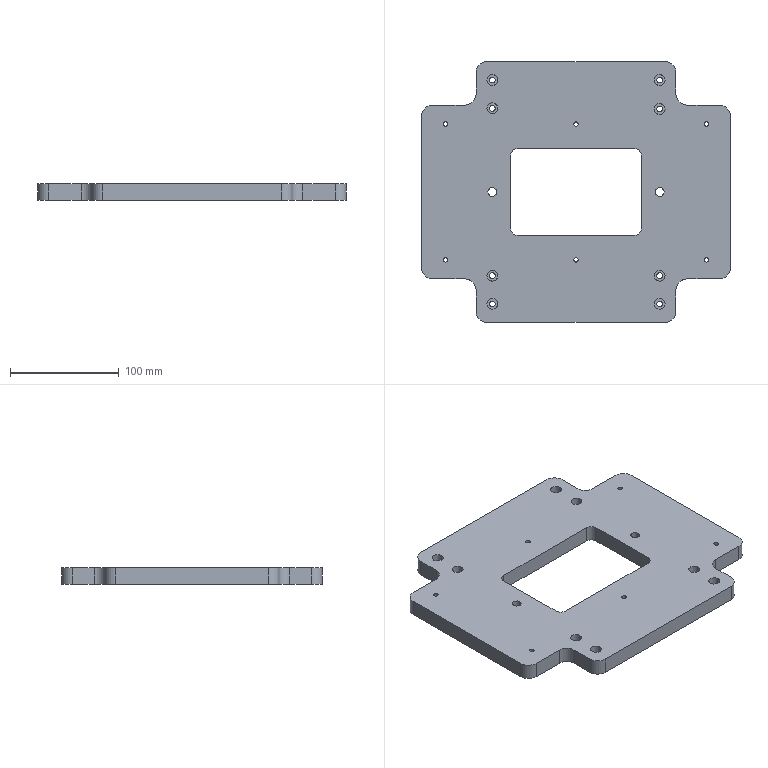CAM job | NX | 3-axis milling, drilling | part box 284 x 240 x 15 mm | stock box 290 x 246 x 15 mm
Tools:
number,name,description,diameter,corner_radius,flute_length,length,flutes
7,D6A45,Milling Tool-5 Parameters,6.0,0.0,50.0,75.0,2
13,5.3ZT,Drilling Tool,5.3,0.0,35.0,50.0,2
12,4.2ZT,Drilling Tool,4.0,0.0,35.0,50.0,2
14,7.8ZT,Drilling Tool,7.8,0.0,35.0,50.0,2
6,D6,Milling Tool-5 Parameters,6.0,0.0,50.0,75.0,2
10,D10,Milling Tool-5 Parameters,10.0,0.0,50.0,75.0,2
9,D10JING,Milling Tool-5 Parameters,10.0,0.0,50.0,75.0,2
Operations:
program,operation,operation_type,tool,method,geometry_group,spindle_rpm,surface_speed,feed_per_tooth,feed_cut,feed_plunge,cut_length_mm,path_length_mm,cut_time_min,machine_time_min
1,DRILLING,Operation,D6A45,METHOD,A,5000.0,94.0,0.025,250.0,0.0,64.0,1084.904,0.256,0.3581
1,DRILLING_COPY,Operation,4.2ZT,METHOD,A,2000.0,33.0,0.05,200.0,0.0,121.21,922.607,0.6061,0.6862
1,DRILLING_COPY_1,Operation,5.3ZT,METHOD,A,2000.0,33.0,0.05,200.0,0.0,164.738,977.25,0.8237,0.9049
1,DRILLING_COPY_COPY,Operation,7.8ZT,METHOD,A,2000.0,33.0,0.05,200.0,0.0,42.687,302.403,0.2134,0.2394
1,HOLE_MILLING_1,CylinderMilling,D6,METHOD,A,9500.0,179.0,0.0842,1600.0,100.0,2666.059,3804.059,1.666,1.78
1,PLANAR_MILL,PlanarMilling,D10,METHOD,A,9500.0,298.0,0.1579,3000.0,1000.0,47732.086,48832.628,16.675,16.785
1,ZLEVEL_PROFILE,ZLevelMilling,D10,METHOD,A,9500.0,298.0,0.1579,3000.0,1000.0,30924.425,30996.325,10.334,10.341
1,ZLEVEL_PROFILE_COPY_COPY,ZLevelMilling,D10JING,METHOD,A,9500.0,298.0,0.0632,1200.0,1000.0,367.504,454.504,0.3071,0.3158
1,ZLEVEL_PROFILE_COPY,ZLevelMilling,D10JING,METHOD,A,9500.0,298.0,0.0632,1200.0,1000.0,1036.373,1123.174,0.8643,0.873
1,PLANAR_MILL_1,PlanarMilling,D6A45,METHOD,A,9500.0,179.0,0.0658,1250.0,100.0,1760.65,3971.192,1.409,1.63
1,刀补6,CylinderMilling,D6,METHOD,A,9500.0,179.0,0.0526,1000.0,100.0,205.567,508.567,0.2056,0.2359